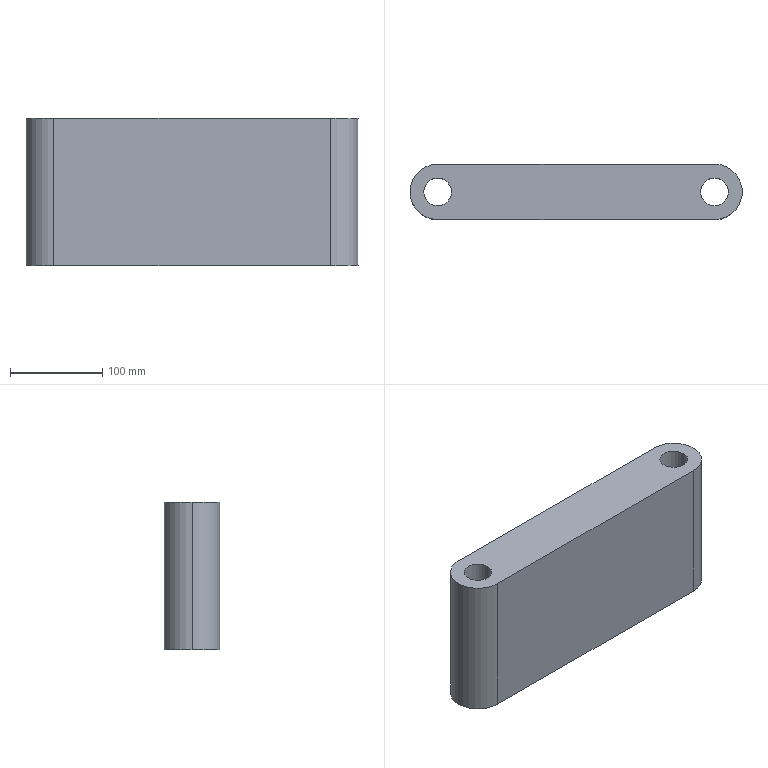Part | SolidWorks | 1 solid | 11 faces | box 360 x 60 x 160 mm | volume 3106195 mm3 | cylinder 7 | plane 4 | commonest cylinder face diameters 30 x4 60 x3
STEP:
#1=CARTESIAN_POINT('',(336.288,-49.56,80.));
#2=VERTEX_POINT('',#1);
#3=CARTESIAN_POINT('',(366.288,-49.56,80.));
#4=VERTEX_POINT('',#3);
#5=CARTESIAN_POINT('',(351.288,-49.56,80.));
#6=DIRECTION('',(0.,0.,1.));
#7=DIRECTION('',(1.,0.,0.));
#8=AXIS2_PLACEMENT_3D('',#5,#6,#7);
#9=CIRCLE('',#8,15.);
#10=EDGE_CURVE('',#2,#4,#9,.T.);
#11=ORIENTED_EDGE('',*,*,#10,.T.);
#12=CARTESIAN_POINT('',(366.288,-49.56,-80.));
#13=VERTEX_POINT('',#12);
#14=CARTESIAN_POINT('',(366.288,-49.56,80.));
#15=DIRECTION('',(0.,0.,-1.));
#16=VECTOR('',#15,1000.);
#17=LINE('',#14,#16);
#18=EDGE_CURVE('',#4,#13,#17,.T.);
#19=ORIENTED_EDGE('',*,*,#18,.T.);
#20=CARTESIAN_POINT('',(336.288,-49.56,-80.));
#21=VERTEX_POINT('',#20);
#22=CARTESIAN_POINT('',(351.288,-49.56,-80.));
#23=DIRECTION('',(0.,0.,1.));
#24=DIRECTION('',(1.,0.,0.));
#25=AXIS2_PLACEMENT_3D('',#22,#23,#24);
#26=CIRCLE('',#25,15.);
#27=EDGE_CURVE('',#21,#13,#26,.T.);
#28=ORIENTED_EDGE('',*,*,#27,.F.);
#29=CARTESIAN_POINT('',(336.288,-49.56,80.));
#30=DIRECTION('',(0.,0.,-1.));
#31=VECTOR('',#30,1000.);
#32=LINE('',#29,#31);
#33=EDGE_CURVE('',#2,#21,#32,.T.);
#34=ORIENTED_EDGE('',*,*,#33,.F.);
#35=EDGE_LOOP('',(#11,#19,#28,#34));
#36=FACE_OUTER_BOUND('',#35,.T.);
#37=CARTESIAN_POINT('',(351.288,-49.56,80.));
#38=DIRECTION('',(0.,0.,-1.));
#39=DIRECTION('',(-1.,0.,0.));
#40=AXIS2_PLACEMENT_3D('',#37,#38,#39);
#41=CYLINDRICAL_SURFACE('',#40,15.);
#42=ADVANCED_FACE('',(#36),#41,.F.);
#43=CARTESIAN_POINT('',(36.288,-49.56,80.));
#44=VERTEX_POINT('',#43);
#45=CARTESIAN_POINT('',(66.288,-49.56,80.));
#46=VERTEX_POINT('',#45);
#47=CARTESIAN_POINT('',(51.288,-49.56,80.));
#48=DIRECTION('',(0.,0.,1.));
#49=DIRECTION('',(1.,0.,0.));
#50=AXIS2_PLACEMENT_3D('',#47,#48,#49);
#51=CIRCLE('',#50,15.);
#52=EDGE_CURVE('',#44,#46,#51,.T.);
#53=ORIENTED_EDGE('',*,*,#52,.T.);
#54=CARTESIAN_POINT('',(66.288,-49.56,-80.));
#55=VERTEX_POINT('',#54);
#56=CARTESIAN_POINT('',(66.288,-49.56,80.));
#57=DIRECTION('',(0.,0.,-1.));
#58=VECTOR('',#57,1000.);
#59=LINE('',#56,#58);
#60=EDGE_CURVE('',#46,#55,#59,.T.);
#61=ORIENTED_EDGE('',*,*,#60,.T.);
#62=CARTESIAN_POINT('',(36.288,-49.56,-80.));
#63=VERTEX_POINT('',#62);
#64=CARTESIAN_POINT('',(51.288,-49.56,-80.));
#65=DIRECTION('',(0.,0.,1.));
#66=DIRECTION('',(1.,0.,0.));
#67=AXIS2_PLACEMENT_3D('',#64,#65,#66);
#68=CIRCLE('',#67,15.);
#69=EDGE_CURVE('',#63,#55,#68,.T.);
#70=ORIENTED_EDGE('',*,*,#69,.F.);
#71=CARTESIAN_POINT('',(36.288,-49.56,80.));
#72=DIRECTION('',(0.,0.,-1.));
#73=VECTOR('',#72,1000.);
#74=LINE('',#71,#73);
#75=EDGE_CURVE('',#44,#63,#74,.T.);
#76=ORIENTED_EDGE('',*,*,#75,.F.);
#77=EDGE_LOOP('',(#53,#61,#70,#76));
#78=FACE_OUTER_BOUND('',#77,.T.);
#79=CARTESIAN_POINT('',(51.288,-49.56,80.));
#80=DIRECTION('',(0.,0.,-1.));
#81=DIRECTION('',(-1.,0.,0.));
#82=AXIS2_PLACEMENT_3D('',#79,#80,#81);
#83=CYLINDRICAL_SURFACE('',#82,15.);
#84=ADVANCED_FACE('',(#78),#83,.F.);
#85=CARTESIAN_POINT('',(21.288,-49.56,80.));
#86=VERTEX_POINT('',#85);
#87=CARTESIAN_POINT('',(51.288,-79.56,80.));
#88=VERTEX_POINT('',#87);
#89=CARTESIAN_POINT('',(51.288,-49.56,80.));
#90=DIRECTION('',(0.,0.,1.));
#91=DIRECTION('',(1.,0.,0.));
#92=AXIS2_PLACEMENT_3D('',#89,#90,#91);
#93=CIRCLE('',#92,30.);
#94=EDGE_CURVE('',#86,#88,#93,.T.);
#95=ORIENTED_EDGE('',*,*,#94,.F.);
#96=CARTESIAN_POINT('',(21.288,-49.56,-80.));
#97=VERTEX_POINT('',#96);
#98=CARTESIAN_POINT('',(21.288,-49.56,80.));
#99=DIRECTION('',(0.,0.,-1.));
#100=VECTOR('',#99,1000.);
#101=LINE('',#98,#100);
#102=EDGE_CURVE('',#86,#97,#101,.T.);
#103=ORIENTED_EDGE('',*,*,#102,.T.);
#104=CARTESIAN_POINT('',(51.288,-79.56,-80.));
#105=VERTEX_POINT('',#104);
#106=CARTESIAN_POINT('',(51.288,-49.56,-80.));
#107=DIRECTION('',(0.,0.,1.));
#108=DIRECTION('',(1.,0.,0.));
#109=AXIS2_PLACEMENT_3D('',#106,#107,#108);
#110=CIRCLE('',#109,30.);
#111=EDGE_CURVE('',#97,#105,#110,.T.);
#112=ORIENTED_EDGE('',*,*,#111,.T.);
#113=CARTESIAN_POINT('',(51.288,-79.56,80.));
#114=DIRECTION('',(0.,0.,-1.));
#115=VECTOR('',#114,1000.);
#116=LINE('',#113,#115);
#117=EDGE_CURVE('',#88,#105,#116,.T.);
#118=ORIENTED_EDGE('',*,*,#117,.F.);
#119=EDGE_LOOP('',(#95,#103,#112,#118));
#120=FACE_OUTER_BOUND('',#119,.T.);
#121=CARTESIAN_POINT('',(51.288,-49.56,80.));
#122=DIRECTION('',(0.,0.,-1.));
#123=DIRECTION('',(-1.,0.,0.));
#124=AXIS2_PLACEMENT_3D('',#121,#122,#123);
#125=CYLINDRICAL_SURFACE('',#124,30.);
#126=ADVANCED_FACE('',(#120),#125,.T.);
#127=ORIENTED_EDGE('',*,*,#52,.F.);
#128=CARTESIAN_POINT('',(51.288,-49.56,80.));
#129=DIRECTION('',(0.,0.,1.));
#130=DIRECTION('',(1.,0.,0.));
#131=AXIS2_PLACEMENT_3D('',#128,#129,#130);
#132=CIRCLE('',#131,15.);
#133=EDGE_CURVE('',#46,#44,#132,.T.);
#134=ORIENTED_EDGE('',*,*,#133,.F.);
#135=EDGE_LOOP('',(#127,#134));
#136=FACE_BOUND('',#135,.T.);
#137=CARTESIAN_POINT('',(51.288,-19.56,80.));
#138=VERTEX_POINT('',#137);
#139=CARTESIAN_POINT('',(51.288,-49.56,80.));
#140=DIRECTION('',(0.,0.,1.));
#141=DIRECTION('',(1.,0.,0.));
#142=AXIS2_PLACEMENT_3D('',#139,#140,#141);
#143=CIRCLE('',#142,30.);
#144=EDGE_CURVE('',#138,#86,#143,.T.);
#145=ORIENTED_EDGE('',*,*,#144,.T.);
#146=ORIENTED_EDGE('',*,*,#94,.T.);
#147=CARTESIAN_POINT('',(351.288,-79.56,80.));
#148=VERTEX_POINT('',#147);
#149=CARTESIAN_POINT('',(51.288,-79.56,80.));
#150=DIRECTION('',(1.,0.,0.));
#151=VECTOR('',#150,1000.);
#152=LINE('',#149,#151);
#153=EDGE_CURVE('',#88,#148,#152,.T.);
#154=ORIENTED_EDGE('',*,*,#153,.T.);
#155=CARTESIAN_POINT('',(351.288,-19.56,80.));
#156=VERTEX_POINT('',#155);
#157=CARTESIAN_POINT('',(351.288,-49.56,80.));
#158=DIRECTION('',(0.,0.,1.));
#159=DIRECTION('',(1.,0.,0.));
#160=AXIS2_PLACEMENT_3D('',#157,#158,#159);
#161=CIRCLE('',#160,30.);
#162=EDGE_CURVE('',#148,#156,#161,.T.);
#163=ORIENTED_EDGE('',*,*,#162,.T.);
#164=CARTESIAN_POINT('',(51.288,-19.56,80.));
#165=DIRECTION('',(-1.,0.,0.));
#166=VECTOR('',#165,1000.);
#167=LINE('',#164,#166);
#168=EDGE_CURVE('',#156,#138,#167,.T.);
#169=ORIENTED_EDGE('',*,*,#168,.T.);
#170=EDGE_LOOP('',(#145,#146,#154,#163,#169));
#171=FACE_OUTER_BOUND('',#170,.T.);
#172=ORIENTED_EDGE('',*,*,#10,.F.);
#173=CARTESIAN_POINT('',(351.288,-49.56,80.));
#174=DIRECTION('',(0.,0.,1.));
#175=DIRECTION('',(1.,0.,0.));
#176=AXIS2_PLACEMENT_3D('',#173,#174,#175);
#177=CIRCLE('',#176,15.);
#178=EDGE_CURVE('',#4,#2,#177,.T.);
#179=ORIENTED_EDGE('',*,*,#178,.F.);
#180=EDGE_LOOP('',(#172,#179));
#181=FACE_BOUND('',#180,.T.);
#182=CARTESIAN_POINT('',(51.288,-49.56,80.));
#183=DIRECTION('',(0.,0.,1.));
#184=DIRECTION('',(1.,0.,0.));
#185=AXIS2_PLACEMENT_3D('',#182,#183,#184);
#186=PLANE('',#185);
#187=ADVANCED_FACE('',(#136,#171,#181),#186,.T.);
#188=CARTESIAN_POINT('',(51.288,-19.56,-80.));
#189=VERTEX_POINT('',#188);
#190=CARTESIAN_POINT('',(51.288,-49.56,-80.));
#191=DIRECTION('',(0.,0.,1.));
#192=DIRECTION('',(1.,0.,0.));
#193=AXIS2_PLACEMENT_3D('',#190,#191,#192);
#194=CIRCLE('',#193,30.);
#195=EDGE_CURVE('',#189,#97,#194,.T.);
#196=ORIENTED_EDGE('',*,*,#195,.F.);
#197=CARTESIAN_POINT('',(351.288,-19.56,-80.));
#198=VERTEX_POINT('',#197);
#199=CARTESIAN_POINT('',(51.288,-19.56,-80.));
#200=DIRECTION('',(-1.,0.,0.));
#201=VECTOR('',#200,1000.);
#202=LINE('',#199,#201);
#203=EDGE_CURVE('',#198,#189,#202,.T.);
#204=ORIENTED_EDGE('',*,*,#203,.F.);
#205=CARTESIAN_POINT('',(351.288,-79.56,-80.));
#206=VERTEX_POINT('',#205);
#207=CARTESIAN_POINT('',(351.288,-49.56,-80.));
#208=DIRECTION('',(0.,0.,1.));
#209=DIRECTION('',(1.,0.,0.));
#210=AXIS2_PLACEMENT_3D('',#207,#208,#209);
#211=CIRCLE('',#210,30.);
#212=EDGE_CURVE('',#206,#198,#211,.T.);
#213=ORIENTED_EDGE('',*,*,#212,.F.);
#214=CARTESIAN_POINT('',(51.288,-79.56,-80.));
#215=DIRECTION('',(1.,0.,0.));
#216=VECTOR('',#215,1000.);
#217=LINE('',#214,#216);
#218=EDGE_CURVE('',#105,#206,#217,.T.);
#219=ORIENTED_EDGE('',*,*,#218,.F.);
#220=ORIENTED_EDGE('',*,*,#111,.F.);
#221=EDGE_LOOP('',(#196,#204,#213,#219,#220));
#222=FACE_OUTER_BOUND('',#221,.T.);
#223=ORIENTED_EDGE('',*,*,#69,.T.);
#224=CARTESIAN_POINT('',(51.288,-49.56,-80.));
#225=DIRECTION('',(0.,0.,1.));
#226=DIRECTION('',(1.,0.,0.));
#227=AXIS2_PLACEMENT_3D('',#224,#225,#226);
#228=CIRCLE('',#227,15.);
#229=EDGE_CURVE('',#55,#63,#228,.T.);
#230=ORIENTED_EDGE('',*,*,#229,.T.);
#231=EDGE_LOOP('',(#223,#230));
#232=FACE_BOUND('',#231,.T.);
#233=ORIENTED_EDGE('',*,*,#27,.T.);
#234=CARTESIAN_POINT('',(351.288,-49.56,-80.));
#235=DIRECTION('',(0.,0.,1.));
#236=DIRECTION('',(1.,0.,0.));
#237=AXIS2_PLACEMENT_3D('',#234,#235,#236);
#238=CIRCLE('',#237,15.);
#239=EDGE_CURVE('',#13,#21,#238,.T.);
#240=ORIENTED_EDGE('',*,*,#239,.T.);
#241=EDGE_LOOP('',(#233,#240));
#242=FACE_BOUND('',#241,.T.);
#243=CARTESIAN_POINT('',(51.288,-49.56,-80.));
#244=DIRECTION('',(0.,0.,1.));
#245=DIRECTION('',(1.,0.,0.));
#246=AXIS2_PLACEMENT_3D('',#243,#244,#245);
#247=PLANE('',#246);
#248=ADVANCED_FACE('',(#222,#232,#242),#247,.F.);
#249=ORIENTED_EDGE('',*,*,#102,.F.);
#250=ORIENTED_EDGE('',*,*,#144,.F.);
#251=CARTESIAN_POINT('',(51.288,-19.56,80.));
#252=DIRECTION('',(0.,0.,-1.));
#253=VECTOR('',#252,1000.);
#254=LINE('',#251,#253);
#255=EDGE_CURVE('',#138,#189,#254,.T.);
#256=ORIENTED_EDGE('',*,*,#255,.T.);
#257=ORIENTED_EDGE('',*,*,#195,.T.);
#258=EDGE_LOOP('',(#249,#250,#256,#257));
#259=FACE_OUTER_BOUND('',#258,.T.);
#260=CARTESIAN_POINT('',(51.288,-49.56,80.));
#261=DIRECTION('',(0.,0.,-1.));
#262=DIRECTION('',(-1.,0.,0.));
#263=AXIS2_PLACEMENT_3D('',#260,#261,#262);
#264=CYLINDRICAL_SURFACE('',#263,30.);
#265=ADVANCED_FACE('',(#259),#264,.T.);
#266=ORIENTED_EDGE('',*,*,#218,.T.);
#267=CARTESIAN_POINT('',(351.288,-79.56,80.));
#268=DIRECTION('',(0.,0.,-1.));
#269=VECTOR('',#268,1000.);
#270=LINE('',#267,#269);
#271=EDGE_CURVE('',#148,#206,#270,.T.);
#272=ORIENTED_EDGE('',*,*,#271,.F.);
#273=ORIENTED_EDGE('',*,*,#153,.F.);
#274=ORIENTED_EDGE('',*,*,#117,.T.);
#275=EDGE_LOOP('',(#266,#272,#273,#274));
#276=FACE_OUTER_BOUND('',#275,.T.);
#277=CARTESIAN_POINT('',(51.288,-79.56,80.));
#278=DIRECTION('',(0.,1.,0.));
#279=DIRECTION('',(0.,0.,1.));
#280=AXIS2_PLACEMENT_3D('',#277,#278,#279);
#281=PLANE('',#280);
#282=ADVANCED_FACE('',(#276),#281,.F.);
#283=ORIENTED_EDGE('',*,*,#212,.T.);
#284=CARTESIAN_POINT('',(351.288,-19.56,80.));
#285=DIRECTION('',(0.,0.,-1.));
#286=VECTOR('',#285,1000.);
#287=LINE('',#284,#286);
#288=EDGE_CURVE('',#156,#198,#287,.T.);
#289=ORIENTED_EDGE('',*,*,#288,.F.);
#290=ORIENTED_EDGE('',*,*,#162,.F.);
#291=ORIENTED_EDGE('',*,*,#271,.T.);
#292=EDGE_LOOP('',(#283,#289,#290,#291));
#293=FACE_OUTER_BOUND('',#292,.T.);
#294=CARTESIAN_POINT('',(351.288,-49.56,80.));
#295=DIRECTION('',(0.,0.,-1.));
#296=DIRECTION('',(-1.,0.,0.));
#297=AXIS2_PLACEMENT_3D('',#294,#295,#296);
#298=CYLINDRICAL_SURFACE('',#297,30.);
#299=ADVANCED_FACE('',(#293),#298,.T.);
#300=ORIENTED_EDGE('',*,*,#203,.T.);
#301=ORIENTED_EDGE('',*,*,#255,.F.);
#302=ORIENTED_EDGE('',*,*,#168,.F.);
#303=ORIENTED_EDGE('',*,*,#288,.T.);
#304=EDGE_LOOP('',(#300,#301,#302,#303));
#305=FACE_OUTER_BOUND('',#304,.T.);
#306=CARTESIAN_POINT('',(51.288,-19.56,80.));
#307=DIRECTION('',(0.,-1.,0.));
#308=DIRECTION('',(0.,0.,-1.));
#309=AXIS2_PLACEMENT_3D('',#306,#307,#308);
#310=PLANE('',#309);
#311=ADVANCED_FACE('',(#305),#310,.F.);
#312=ORIENTED_EDGE('',*,*,#60,.F.);
#313=ORIENTED_EDGE('',*,*,#133,.T.);
#314=ORIENTED_EDGE('',*,*,#75,.T.);
#315=ORIENTED_EDGE('',*,*,#229,.F.);
#316=EDGE_LOOP('',(#312,#313,#314,#315));
#317=FACE_OUTER_BOUND('',#316,.T.);
#318=CARTESIAN_POINT('',(51.288,-49.56,80.));
#319=DIRECTION('',(0.,0.,-1.));
#320=DIRECTION('',(-1.,0.,0.));
#321=AXIS2_PLACEMENT_3D('',#318,#319,#320);
#322=CYLINDRICAL_SURFACE('',#321,15.);
#323=ADVANCED_FACE('',(#317),#322,.F.);
#324=ORIENTED_EDGE('',*,*,#18,.F.);
#325=ORIENTED_EDGE('',*,*,#178,.T.);
#326=ORIENTED_EDGE('',*,*,#33,.T.);
#327=ORIENTED_EDGE('',*,*,#239,.F.);
#328=EDGE_LOOP('',(#324,#325,#326,#327));
#329=FACE_OUTER_BOUND('',#328,.T.);
#330=CARTESIAN_POINT('',(351.288,-49.56,80.));
#331=DIRECTION('',(0.,0.,-1.));
#332=DIRECTION('',(-1.,0.,0.));
#333=AXIS2_PLACEMENT_3D('',#330,#331,#332);
#334=CYLINDRICAL_SURFACE('',#333,15.);
#335=ADVANCED_FACE('',(#329),#334,.F.);
#336=CLOSED_SHELL('',(#42,#84,#126,#187,#248,#265,#282,#299,#311,#323,#335));
#337=MANIFOLD_SOLID_BREP('',#336);
#338=CARTESIAN_POINT('',(0.,0.,0.));
#339=DIRECTION('',(0.,0.,1.));
#340=DIRECTION('',(1.,0.,0.));
#341=AXIS2_PLACEMENT_3D('',#338,#339,#340);
#342=(LENGTH_UNIT()NAMED_UNIT(*)SI_UNIT(.MILLI.,.METRE.));
#343=UNCERTAINTY_MEASURE_WITH_UNIT(LENGTH_MEASURE(0.00001),#342,'','');
#344=(NAMED_UNIT(*)PLANE_ANGLE_UNIT()SI_UNIT($,.RADIAN.));
#345=(NAMED_UNIT(*)SI_UNIT($,.STERADIAN.)SOLID_ANGLE_UNIT());
#346=(GEOMETRIC_REPRESENTATION_CONTEXT(3)GLOBAL_UNCERTAINTY_ASSIGNED_CONTEXT((#343))GLOBAL_UNIT_ASSIGNED_CONTEXT((#342,#344,#345))REPRESENTATION_CONTEXT('',''));
#347=ADVANCED_BREP_SHAPE_REPRESENTATION('',(#337,#341),#346);